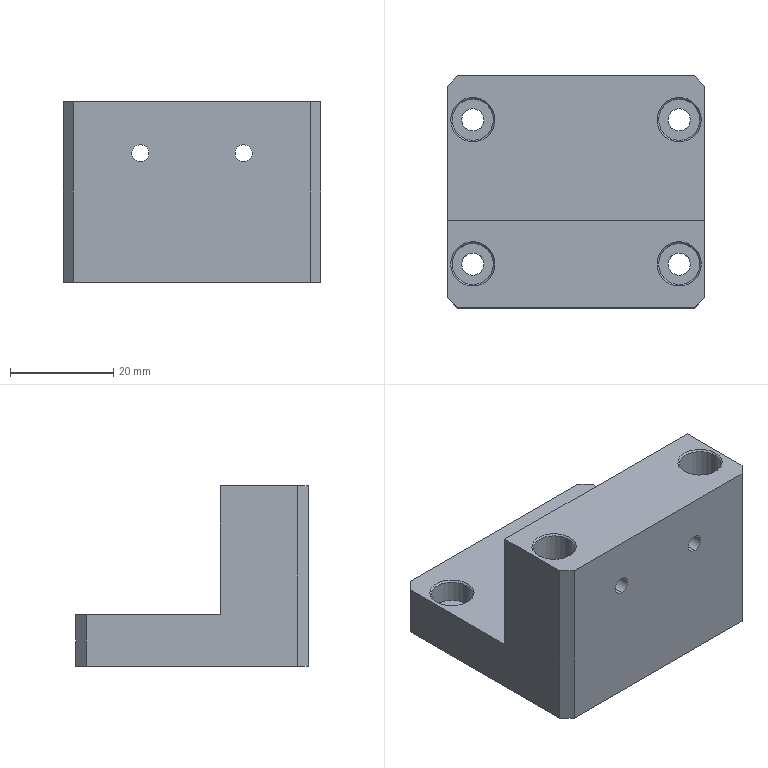Part | SolidWorks | features HoleWzd 3, Chamfer 1, Extrusion 1, ICE 1 | 1 solid | 48 faces | box 50 x 45 x 35 mm | volume 39850 mm3 | cylinder 20 | plane 16 | cone 12 | commonest cylinder face diameters 4.3 x8 8 x8 3.3 x4
STEP:
#1=CARTESIAN_POINT('',(-35.,16.625,23.35));
#2=VERTEX_POINT('',#1);
#3=CARTESIAN_POINT('',(-35.,16.625,26.65));
#4=VERTEX_POINT('',#3);
#5=CARTESIAN_POINT('',(-35.,16.625,25.));
#6=DIRECTION('',(0.,1.,0.));
#7=DIRECTION('',(0.,0.,1.));
#8=AXIS2_PLACEMENT_3D('',#5,#6,#7);
#9=CIRCLE('',#8,1.65);
#10=EDGE_CURVE('',#2,#4,#9,.T.);
#11=ORIENTED_EDGE('',*,*,#10,.F.);
#12=CARTESIAN_POINT('',(-35.,17.,22.975));
#13=VERTEX_POINT('',#12);
#14=CARTESIAN_POINT('',(-35.,17.,22.975));
#15=DIRECTION('',(0.,0.7071,-0.7071));
#16=VECTOR('',#15,1000.);
#17=LINE('',#14,#16);
#18=EDGE_CURVE('',#2,#13,#17,.T.);
#19=ORIENTED_EDGE('',*,*,#18,.T.);
#20=CARTESIAN_POINT('',(-35.,17.,27.025));
#21=VERTEX_POINT('',#20);
#22=CARTESIAN_POINT('',(-35.,17.,25.));
#23=DIRECTION('',(0.,1.,0.));
#24=DIRECTION('',(0.,0.,1.));
#25=AXIS2_PLACEMENT_3D('',#22,#23,#24);
#26=CIRCLE('',#25,2.025);
#27=EDGE_CURVE('',#13,#21,#26,.T.);
#28=ORIENTED_EDGE('',*,*,#27,.T.);
#29=CARTESIAN_POINT('',(-35.,17.,27.025));
#30=DIRECTION('',(0.,0.7071,0.7071));
#31=VECTOR('',#30,1000.);
#32=LINE('',#29,#31);
#33=EDGE_CURVE('',#4,#21,#32,.T.);
#34=ORIENTED_EDGE('',*,*,#33,.F.);
#35=EDGE_LOOP('',(#11,#19,#28,#34));
#36=FACE_OUTER_BOUND('',#35,.T.);
#37=CARTESIAN_POINT('',(-35.,17.,25.));
#38=DIRECTION('',(0.,1.,0.));
#39=DIRECTION('',(0.,0.,1.));
#40=AXIS2_PLACEMENT_3D('',#37,#38,#39);
#41=CONICAL_SURFACE('',#40,2.025,0.7854);
#42=ADVANCED_FACE('',(#36),#41,.F.);
#43=CARTESIAN_POINT('',(-35.,0.,23.35));
#44=VERTEX_POINT('',#43);
#45=CARTESIAN_POINT('',(-35.,0.,26.65));
#46=VERTEX_POINT('',#45);
#47=CARTESIAN_POINT('',(-35.,0.,25.));
#48=DIRECTION('',(0.,1.,0.));
#49=DIRECTION('',(0.,0.,1.));
#50=AXIS2_PLACEMENT_3D('',#47,#48,#49);
#51=CIRCLE('',#50,1.65);
#52=EDGE_CURVE('',#44,#46,#51,.T.);
#53=ORIENTED_EDGE('',*,*,#52,.F.);
#54=CARTESIAN_POINT('',(-35.,17.,23.35));
#55=DIRECTION('',(0.,1.,0.));
#56=VECTOR('',#55,1000.);
#57=LINE('',#54,#56);
#58=EDGE_CURVE('',#44,#2,#57,.T.);
#59=ORIENTED_EDGE('',*,*,#58,.T.);
#60=ORIENTED_EDGE('',*,*,#10,.T.);
#61=CARTESIAN_POINT('',(-35.,17.,26.65));
#62=DIRECTION('',(0.,1.,0.));
#63=VECTOR('',#62,1000.);
#64=LINE('',#61,#63);
#65=EDGE_CURVE('',#46,#4,#64,.T.);
#66=ORIENTED_EDGE('',*,*,#65,.F.);
#67=EDGE_LOOP('',(#53,#59,#60,#66));
#68=FACE_OUTER_BOUND('',#67,.T.);
#69=CARTESIAN_POINT('',(-35.,17.,25.));
#70=DIRECTION('',(0.,1.,0.));
#71=DIRECTION('',(0.,0.,1.));
#72=AXIS2_PLACEMENT_3D('',#69,#70,#71);
#73=CYLINDRICAL_SURFACE('',#72,1.65);
#74=ADVANCED_FACE('',(#68),#73,.F.);
#75=CARTESIAN_POINT('',(-15.,16.625,23.35));
#76=VERTEX_POINT('',#75);
#77=CARTESIAN_POINT('',(-15.,16.625,26.65));
#78=VERTEX_POINT('',#77);
#79=CARTESIAN_POINT('',(-15.,16.625,25.));
#80=DIRECTION('',(0.,1.,0.));
#81=DIRECTION('',(0.,0.,1.));
#82=AXIS2_PLACEMENT_3D('',#79,#80,#81);
#83=CIRCLE('',#82,1.65);
#84=EDGE_CURVE('',#76,#78,#83,.T.);
#85=ORIENTED_EDGE('',*,*,#84,.F.);
#86=CARTESIAN_POINT('',(-15.,17.,22.975));
#87=VERTEX_POINT('',#86);
#88=CARTESIAN_POINT('',(-15.,17.,22.975));
#89=DIRECTION('',(0.,0.7071,-0.7071));
#90=VECTOR('',#89,1000.);
#91=LINE('',#88,#90);
#92=EDGE_CURVE('',#76,#87,#91,.T.);
#93=ORIENTED_EDGE('',*,*,#92,.T.);
#94=CARTESIAN_POINT('',(-15.,17.,27.025));
#95=VERTEX_POINT('',#94);
#96=CARTESIAN_POINT('',(-15.,17.,25.));
#97=DIRECTION('',(0.,1.,0.));
#98=DIRECTION('',(0.,0.,1.));
#99=AXIS2_PLACEMENT_3D('',#96,#97,#98);
#100=CIRCLE('',#99,2.025);
#101=EDGE_CURVE('',#87,#95,#100,.T.);
#102=ORIENTED_EDGE('',*,*,#101,.T.);
#103=CARTESIAN_POINT('',(-15.,17.,27.025));
#104=DIRECTION('',(0.,0.7071,0.7071));
#105=VECTOR('',#104,1000.);
#106=LINE('',#103,#105);
#107=EDGE_CURVE('',#78,#95,#106,.T.);
#108=ORIENTED_EDGE('',*,*,#107,.F.);
#109=EDGE_LOOP('',(#85,#93,#102,#108));
#110=FACE_OUTER_BOUND('',#109,.T.);
#111=CARTESIAN_POINT('',(-15.,17.,25.));
#112=DIRECTION('',(0.,1.,0.));
#113=DIRECTION('',(0.,0.,1.));
#114=AXIS2_PLACEMENT_3D('',#111,#112,#113);
#115=CONICAL_SURFACE('',#114,2.025,0.7854);
#116=ADVANCED_FACE('',(#110),#115,.F.);
#117=CARTESIAN_POINT('',(-15.,0.,23.35));
#118=VERTEX_POINT('',#117);
#119=CARTESIAN_POINT('',(-15.,0.,26.65));
#120=VERTEX_POINT('',#119);
#121=CARTESIAN_POINT('',(-15.,0.,25.));
#122=DIRECTION('',(0.,1.,0.));
#123=DIRECTION('',(0.,0.,1.));
#124=AXIS2_PLACEMENT_3D('',#121,#122,#123);
#125=CIRCLE('',#124,1.65);
#126=EDGE_CURVE('',#118,#120,#125,.T.);
#127=ORIENTED_EDGE('',*,*,#126,.F.);
#128=CARTESIAN_POINT('',(-15.,17.,23.35));
#129=DIRECTION('',(0.,1.,0.));
#130=VECTOR('',#129,1000.);
#131=LINE('',#128,#130);
#132=EDGE_CURVE('',#118,#76,#131,.T.);
#133=ORIENTED_EDGE('',*,*,#132,.T.);
#134=ORIENTED_EDGE('',*,*,#84,.T.);
#135=CARTESIAN_POINT('',(-15.,17.,26.65));
#136=DIRECTION('',(0.,1.,0.));
#137=VECTOR('',#136,1000.);
#138=LINE('',#135,#137);
#139=EDGE_CURVE('',#120,#78,#138,.T.);
#140=ORIENTED_EDGE('',*,*,#139,.F.);
#141=EDGE_LOOP('',(#127,#133,#134,#140));
#142=FACE_OUTER_BOUND('',#141,.T.);
#143=CARTESIAN_POINT('',(-15.,17.,25.));
#144=DIRECTION('',(0.,1.,0.));
#145=DIRECTION('',(0.,0.,1.));
#146=AXIS2_PLACEMENT_3D('',#143,#144,#145);
#147=CYLINDRICAL_SURFACE('',#146,1.65);
#148=ADVANCED_FACE('',(#142),#147,.F.);
#149=CARTESIAN_POINT('',(-49.,8.5,34.7));
#150=VERTEX_POINT('',#149);
#151=CARTESIAN_POINT('',(-41.,8.5,34.7));
#152=VERTEX_POINT('',#151);
#153=CARTESIAN_POINT('',(-45.,8.5,34.7));
#154=DIRECTION('',(0.,0.,1.));
#155=DIRECTION('',(1.,0.,0.));
#156=AXIS2_PLACEMENT_3D('',#153,#154,#155);
#157=CIRCLE('',#156,4.);
#158=EDGE_CURVE('',#150,#152,#157,.T.);
#159=ORIENTED_EDGE('',*,*,#158,.F.);
#160=CARTESIAN_POINT('',(-49.3,8.5,35.));
#161=VERTEX_POINT('',#160);
#162=CARTESIAN_POINT('',(-49.3,8.5,35.));
#163=DIRECTION('',(-0.7071,0.,0.7071));
#164=VECTOR('',#163,1000.);
#165=LINE('',#162,#164);
#166=EDGE_CURVE('',#150,#161,#165,.T.);
#167=ORIENTED_EDGE('',*,*,#166,.T.);
#168=CARTESIAN_POINT('',(-40.7,8.5,35.));
#169=VERTEX_POINT('',#168);
#170=CARTESIAN_POINT('',(-45.,8.5,35.));
#171=DIRECTION('',(0.,0.,1.));
#172=DIRECTION('',(1.,0.,0.));
#173=AXIS2_PLACEMENT_3D('',#170,#171,#172);
#174=CIRCLE('',#173,4.3);
#175=EDGE_CURVE('',#161,#169,#174,.T.);
#176=ORIENTED_EDGE('',*,*,#175,.T.);
#177=CARTESIAN_POINT('',(-40.7,8.5,35.));
#178=DIRECTION('',(0.7071,0.,0.7071));
#179=VECTOR('',#178,1000.);
#180=LINE('',#177,#179);
#181=EDGE_CURVE('',#152,#169,#180,.T.);
#182=ORIENTED_EDGE('',*,*,#181,.F.);
#183=EDGE_LOOP('',(#159,#167,#176,#182));
#184=FACE_OUTER_BOUND('',#183,.T.);
#185=CARTESIAN_POINT('',(-45.,8.5,35.));
#186=DIRECTION('',(0.,0.,1.));
#187=DIRECTION('',(1.,0.,0.));
#188=AXIS2_PLACEMENT_3D('',#185,#186,#187);
#189=CONICAL_SURFACE('',#188,4.3,0.7854);
#190=ADVANCED_FACE('',(#184),#189,.F.);
#191=CARTESIAN_POINT('',(-49.,8.5,10.));
#192=VERTEX_POINT('',#191);
#193=CARTESIAN_POINT('',(-41.,8.5,10.));
#194=VERTEX_POINT('',#193);
#195=CARTESIAN_POINT('',(-45.,8.5,10.));
#196=DIRECTION('',(0.,0.,1.));
#197=DIRECTION('',(1.,0.,0.));
#198=AXIS2_PLACEMENT_3D('',#195,#196,#197);
#199=CIRCLE('',#198,4.);
#200=EDGE_CURVE('',#192,#194,#199,.T.);
#201=ORIENTED_EDGE('',*,*,#200,.F.);
#202=CARTESIAN_POINT('',(-49.,8.5,35.));
#203=DIRECTION('',(0.,0.,1.));
#204=VECTOR('',#203,1000.);
#205=LINE('',#202,#204);
#206=EDGE_CURVE('',#192,#150,#205,.T.);
#207=ORIENTED_EDGE('',*,*,#206,.T.);
#208=ORIENTED_EDGE('',*,*,#158,.T.);
#209=CARTESIAN_POINT('',(-41.,8.5,35.));
#210=DIRECTION('',(0.,0.,1.));
#211=VECTOR('',#210,1000.);
#212=LINE('',#209,#211);
#213=EDGE_CURVE('',#194,#152,#212,.T.);
#214=ORIENTED_EDGE('',*,*,#213,.F.);
#215=EDGE_LOOP('',(#201,#207,#208,#214));
#216=FACE_OUTER_BOUND('',#215,.T.);
#217=CARTESIAN_POINT('',(-45.,8.5,35.));
#218=DIRECTION('',(0.,0.,1.));
#219=DIRECTION('',(1.,0.,0.));
#220=AXIS2_PLACEMENT_3D('',#217,#218,#219);
#221=CYLINDRICAL_SURFACE('',#220,4.);
#222=ADVANCED_FACE('',(#216),#221,.F.);
#223=CARTESIAN_POINT('',(-47.15,8.5,0.));
#224=VERTEX_POINT('',#223);
#225=CARTESIAN_POINT('',(-42.85,8.5,0.));
#226=VERTEX_POINT('',#225);
#227=CARTESIAN_POINT('',(-45.,8.5,0.));
#228=DIRECTION('',(0.,0.,1.));
#229=DIRECTION('',(1.,0.,0.));
#230=AXIS2_PLACEMENT_3D('',#227,#228,#229);
#231=CIRCLE('',#230,2.15);
#232=EDGE_CURVE('',#224,#226,#231,.T.);
#233=ORIENTED_EDGE('',*,*,#232,.F.);
#234=CARTESIAN_POINT('',(-47.15,8.5,10.));
#235=VERTEX_POINT('',#234);
#236=CARTESIAN_POINT('',(-47.15,8.5,35.));
#237=DIRECTION('',(0.,0.,1.));
#238=VECTOR('',#237,1000.);
#239=LINE('',#236,#238);
#240=EDGE_CURVE('',#224,#235,#239,.T.);
#241=ORIENTED_EDGE('',*,*,#240,.T.);
#242=CARTESIAN_POINT('',(-42.85,8.5,10.));
#243=VERTEX_POINT('',#242);
#244=CARTESIAN_POINT('',(-45.,8.5,10.));
#245=DIRECTION('',(0.,0.,1.));
#246=DIRECTION('',(1.,0.,0.));
#247=AXIS2_PLACEMENT_3D('',#244,#245,#246);
#248=CIRCLE('',#247,2.15);
#249=EDGE_CURVE('',#235,#243,#248,.T.);
#250=ORIENTED_EDGE('',*,*,#249,.T.);
#251=CARTESIAN_POINT('',(-42.85,8.5,35.));
#252=DIRECTION('',(0.,0.,1.));
#253=VECTOR('',#252,1000.);
#254=LINE('',#251,#253);
#255=EDGE_CURVE('',#226,#243,#254,.T.);
#256=ORIENTED_EDGE('',*,*,#255,.F.);
#257=EDGE_LOOP('',(#233,#241,#250,#256));
#258=FACE_OUTER_BOUND('',#257,.T.);
#259=CARTESIAN_POINT('',(-45.,8.5,35.));
#260=DIRECTION('',(0.,0.,1.));
#261=DIRECTION('',(1.,0.,0.));
#262=AXIS2_PLACEMENT_3D('',#259,#260,#261);
#263=CYLINDRICAL_SURFACE('',#262,2.15);
#264=ADVANCED_FACE('',(#258),#263,.F.);
#265=CARTESIAN_POINT('',(-9.,8.5,34.7));
#266=VERTEX_POINT('',#265);
#267=CARTESIAN_POINT('',(-1.,8.5,34.7));
#268=VERTEX_POINT('',#267);
#269=CARTESIAN_POINT('',(-5.,8.5,34.7));
#270=DIRECTION('',(0.,0.,1.));
#271=DIRECTION('',(1.,0.,0.));
#272=AXIS2_PLACEMENT_3D('',#269,#270,#271);
#273=CIRCLE('',#272,4.);
#274=EDGE_CURVE('',#266,#268,#273,.T.);
#275=ORIENTED_EDGE('',*,*,#274,.F.);
#276=CARTESIAN_POINT('',(-9.3,8.5,35.));
#277=VERTEX_POINT('',#276);
#278=CARTESIAN_POINT('',(-9.3,8.5,35.));
#279=DIRECTION('',(-0.7071,0.,0.7071));
#280=VECTOR('',#279,1000.);
#281=LINE('',#278,#280);
#282=EDGE_CURVE('',#266,#277,#281,.T.);
#283=ORIENTED_EDGE('',*,*,#282,.T.);
#284=CARTESIAN_POINT('',(-0.7,8.5,35.));
#285=VERTEX_POINT('',#284);
#286=CARTESIAN_POINT('',(-5.,8.5,35.));
#287=DIRECTION('',(0.,0.,1.));
#288=DIRECTION('',(1.,0.,0.));
#289=AXIS2_PLACEMENT_3D('',#286,#287,#288);
#290=CIRCLE('',#289,4.3);
#291=EDGE_CURVE('',#277,#285,#290,.T.);
#292=ORIENTED_EDGE('',*,*,#291,.T.);
#293=CARTESIAN_POINT('',(-0.7,8.5,35.));
#294=DIRECTION('',(0.7071,0.,0.7071));
#295=VECTOR('',#294,1000.);
#296=LINE('',#293,#295);
#297=EDGE_CURVE('',#268,#285,#296,.T.);
#298=ORIENTED_EDGE('',*,*,#297,.F.);
#299=EDGE_LOOP('',(#275,#283,#292,#298));
#300=FACE_OUTER_BOUND('',#299,.T.);
#301=CARTESIAN_POINT('',(-5.,8.5,35.));
#302=DIRECTION('',(0.,0.,1.));
#303=DIRECTION('',(1.,0.,0.));
#304=AXIS2_PLACEMENT_3D('',#301,#302,#303);
#305=CONICAL_SURFACE('',#304,4.3,0.7854);
#306=ADVANCED_FACE('',(#300),#305,.F.);
#307=CARTESIAN_POINT('',(-9.,8.5,10.));
#308=VERTEX_POINT('',#307);
#309=CARTESIAN_POINT('',(-1.,8.5,10.));
#310=VERTEX_POINT('',#309);
#311=CARTESIAN_POINT('',(-5.,8.5,10.));
#312=DIRECTION('',(0.,0.,1.));
#313=DIRECTION('',(1.,0.,0.));
#314=AXIS2_PLACEMENT_3D('',#311,#312,#313);
#315=CIRCLE('',#314,4.);
#316=EDGE_CURVE('',#308,#310,#315,.T.);
#317=ORIENTED_EDGE('',*,*,#316,.F.);
#318=CARTESIAN_POINT('',(-9.,8.5,35.));
#319=DIRECTION('',(0.,0.,1.));
#320=VECTOR('',#319,1000.);
#321=LINE('',#318,#320);
#322=EDGE_CURVE('',#308,#266,#321,.T.);
#323=ORIENTED_EDGE('',*,*,#322,.T.);
#324=ORIENTED_EDGE('',*,*,#274,.T.);
#325=CARTESIAN_POINT('',(-1.,8.5,35.));
#326=DIRECTION('',(0.,0.,1.));
#327=VECTOR('',#326,1000.);
#328=LINE('',#325,#327);
#329=EDGE_CURVE('',#310,#268,#328,.T.);
#330=ORIENTED_EDGE('',*,*,#329,.F.);
#331=EDGE_LOOP('',(#317,#323,#324,#330));
#332=FACE_OUTER_BOUND('',#331,.T.);
#333=CARTESIAN_POINT('',(-5.,8.5,35.));
#334=DIRECTION('',(0.,0.,1.));
#335=DIRECTION('',(1.,0.,0.));
#336=AXIS2_PLACEMENT_3D('',#333,#334,#335);
#337=CYLINDRICAL_SURFACE('',#336,4.);
#338=ADVANCED_FACE('',(#332),#337,.F.);
#339=CARTESIAN_POINT('',(-7.15,8.5,0.));
#340=VERTEX_POINT('',#339);
#341=CARTESIAN_POINT('',(-2.85,8.5,0.));
#342=VERTEX_POINT('',#341);
#343=CARTESIAN_POINT('',(-5.,8.5,0.));
#344=DIRECTION('',(0.,0.,1.));
#345=DIRECTION('',(1.,0.,0.));
#346=AXIS2_PLACEMENT_3D('',#343,#344,#345);
#347=CIRCLE('',#346,2.15);
#348=EDGE_CURVE('',#340,#342,#347,.T.);
#349=ORIENTED_EDGE('',*,*,#348,.F.);
#350=CARTESIAN_POINT('',(-7.15,8.5,10.));
#351=VERTEX_POINT('',#350);
#352=CARTESIAN_POINT('',(-7.15,8.5,35.));
#353=DIRECTION('',(0.,0.,1.));
#354=VECTOR('',#353,1000.);
#355=LINE('',#352,#354);
#356=EDGE_CURVE('',#340,#351,#355,.T.);
#357=ORIENTED_EDGE('',*,*,#356,.T.);
#358=CARTESIAN_POINT('',(-2.85,8.5,10.));
#359=VERTEX_POINT('',#358);
#360=CARTESIAN_POINT('',(-5.,8.5,10.));
#361=DIRECTION('',(0.,0.,1.));
#362=DIRECTION('',(1.,0.,0.));
#363=AXIS2_PLACEMENT_3D('',#360,#361,#362);
#364=CIRCLE('',#363,2.15);
#365=EDGE_CURVE('',#351,#359,#364,.T.);
#366=ORIENTED_EDGE('',*,*,#365,.T.);
#367=CARTESIAN_POINT('',(-2.85,8.5,35.));
#368=DIRECTION('',(0.,0.,1.));
#369=VECTOR('',#368,1000.);
#370=LINE('',#367,#369);
#371=EDGE_CURVE('',#342,#359,#370,.T.);
#372=ORIENTED_EDGE('',*,*,#371,.F.);
#373=EDGE_LOOP('',(#349,#357,#366,#372));
#374=FACE_OUTER_BOUND('',#373,.T.);
#375=CARTESIAN_POINT('',(-5.,8.5,35.));
#376=DIRECTION('',(0.,0.,1.));
#377=DIRECTION('',(1.,0.,0.));
#378=AXIS2_PLACEMENT_3D('',#375,#376,#377);
#379=CYLINDRICAL_SURFACE('',#378,2.15);
#380=ADVANCED_FACE('',(#374),#379,.F.);
#381=CARTESIAN_POINT('',(-49.,36.5,9.7));
#382=VERTEX_POINT('',#381);
#383=CARTESIAN_POINT('',(-41.,36.5,9.7));
#384=VERTEX_POINT('',#383);
#385=CARTESIAN_POINT('',(-45.,36.5,9.7));
#386=DIRECTION('',(0.,0.,1.));
#387=DIRECTION('',(1.,0.,0.));
#388=AXIS2_PLACEMENT_3D('',#385,#386,#387);
#389=CIRCLE('',#388,4.);
#390=EDGE_CURVE('',#382,#384,#389,.T.);
#391=ORIENTED_EDGE('',*,*,#390,.F.);
#392=CARTESIAN_POINT('',(-49.3,36.5,10.));
#393=VERTEX_POINT('',#392);
#394=CARTESIAN_POINT('',(-49.3,36.5,10.));
#395=DIRECTION('',(-0.7071,0.,0.7071));
#396=VECTOR('',#395,1000.);
#397=LINE('',#394,#396);
#398=EDGE_CURVE('',#382,#393,#397,.T.);
#399=ORIENTED_EDGE('',*,*,#398,.T.);
#400=CARTESIAN_POINT('',(-40.7,36.5,10.));
#401=VERTEX_POINT('',#400);
#402=CARTESIAN_POINT('',(-45.,36.5,10.));
#403=DIRECTION('',(0.,0.,1.));
#404=DIRECTION('',(1.,0.,0.));
#405=AXIS2_PLACEMENT_3D('',#402,#403,#404);
#406=CIRCLE('',#405,4.3);
#407=EDGE_CURVE('',#393,#401,#406,.T.);
#408=ORIENTED_EDGE('',*,*,#407,.T.);
#409=CARTESIAN_POINT('',(-40.7,36.5,10.));
#410=DIRECTION('',(0.7071,0.,0.7071));
#411=VECTOR('',#410,1000.);
#412=LINE('',#409,#411);
#413=EDGE_CURVE('',#384,#401,#412,.T.);
#414=ORIENTED_EDGE('',*,*,#413,.F.);
#415=EDGE_LOOP('',(#391,#399,#408,#414));
#416=FACE_OUTER_BOUND('',#415,.T.);
#417=CARTESIAN_POINT('',(-45.,36.5,10.));
#418=DIRECTION('',(0.,0.,1.));
#419=DIRECTION('',(1.,0.,0.));
#420=AXIS2_PLACEMENT_3D('',#417,#418,#419);
#421=CONICAL_SURFACE('',#420,4.3,0.7854);
#422=ADVANCED_FACE('',(#416),#421,.F.);
#423=CARTESIAN_POINT('',(-49.,36.5,5.4));
#424=VERTEX_POINT('',#423);
#425=CARTESIAN_POINT('',(-41.,36.5,5.4));
#426=VERTEX_POINT('',#425);
#427=CARTESIAN_POINT('',(-45.,36.5,5.4));
#428=DIRECTION('',(0.,0.,1.));
#429=DIRECTION('',(1.,0.,0.));
#430=AXIS2_PLACEMENT_3D('',#427,#428,#429);
#431=CIRCLE('',#430,4.);
#432=EDGE_CURVE('',#424,#426,#431,.T.);
#433=ORIENTED_EDGE('',*,*,#432,.F.);
#434=CARTESIAN_POINT('',(-49.,36.5,10.));
#435=DIRECTION('',(0.,0.,1.));
#436=VECTOR('',#435,1000.);
#437=LINE('',#434,#436);
#438=EDGE_CURVE('',#424,#382,#437,.T.);
#439=ORIENTED_EDGE('',*,*,#438,.T.);
#440=ORIENTED_EDGE('',*,*,#390,.T.);
#441=CARTESIAN_POINT('',(-41.,36.5,10.));
#442=DIRECTION('',(0.,0.,1.));
#443=VECTOR('',#442,1000.);
#444=LINE('',#441,#443);
#445=EDGE_CURVE('',#426,#384,#444,.T.);
#446=ORIENTED_EDGE('',*,*,#445,.F.);
#447=EDGE_LOOP('',(#433,#439,#440,#446));
#448=FACE_OUTER_BOUND('',#447,.T.);
#449=CARTESIAN_POINT('',(-45.,36.5,10.));
#450=DIRECTION('',(0.,0.,1.));
#451=DIRECTION('',(1.,0.,0.));
#452=AXIS2_PLACEMENT_3D('',#449,#450,#451);
#453=CYLINDRICAL_SURFACE('',#452,4.);
#454=ADVANCED_FACE('',(#448),#453,.F.);
#455=CARTESIAN_POINT('',(-47.15,36.5,0.));
#456=VERTEX_POINT('',#455);
#457=CARTESIAN_POINT('',(-42.85,36.5,0.));
#458=VERTEX_POINT('',#457);
#459=CARTESIAN_POINT('',(-45.,36.5,0.));
#460=DIRECTION('',(0.,0.,1.));
#461=DIRECTION('',(1.,0.,0.));
#462=AXIS2_PLACEMENT_3D('',#459,#460,#461);
#463=CIRCLE('',#462,2.15);
#464=EDGE_CURVE('',#456,#458,#463,.T.);
#465=ORIENTED_EDGE('',*,*,#464,.F.);
#466=CARTESIAN_POINT('',(-47.15,36.5,5.4));
#467=VERTEX_POINT('',#466);
#468=CARTESIAN_POINT('',(-47.15,36.5,10.));
#469=DIRECTION('',(0.,0.,1.));
#470=VECTOR('',#469,1000.);
#471=LINE('',#468,#470);
#472=EDGE_CURVE('',#456,#467,#471,.T.);
#473=ORIENTED_EDGE('',*,*,#472,.T.);
#474=CARTESIAN_POINT('',(-42.85,36.5,5.4));
#475=VERTEX_POINT('',#474);
#476=CARTESIAN_POINT('',(-45.,36.5,5.4));
#477=DIRECTION('',(0.,0.,1.));
#478=DIRECTION('',(1.,0.,0.));
#479=AXIS2_PLACEMENT_3D('',#476,#477,#478);
#480=CIRCLE('',#479,2.15);
#481=EDGE_CURVE('',#467,#475,#480,.T.);
#482=ORIENTED_EDGE('',*,*,#481,.T.);
#483=CARTESIAN_POINT('',(-42.85,36.5,10.));
#484=DIRECTION('',(0.,0.,1.));
#485=VECTOR('',#484,1000.);
#486=LINE('',#483,#485);
#487=EDGE_CURVE('',#458,#475,#486,.T.);
#488=ORIENTED_EDGE('',*,*,#487,.F.);
#489=EDGE_LOOP('',(#465,#473,#482,#488));
#490=FACE_OUTER_BOUND('',#489,.T.);
#491=CARTESIAN_POINT('',(-45.,36.5,10.));
#492=DIRECTION('',(0.,0.,1.));
#493=DIRECTION('',(1.,0.,0.));
#494=AXIS2_PLACEMENT_3D('',#491,#492,#493);
#495=CYLINDRICAL_SURFACE('',#494,2.15);
#496=ADVANCED_FACE('',(#490),#495,.F.);
#497=CARTESIAN_POINT('',(-9.,36.5,9.7));
#498=VERTEX_POINT('',#497);
#499=CARTESIAN_POINT('',(-1.,36.5,9.7));
#500=VERTEX_POINT('',#499);
#501=CARTESIAN_POINT('',(-5.,36.5,9.7));
#502=DIRECTION('',(0.,0.,1.));
#503=DIRECTION('',(1.,0.,0.));
#504=AXIS2_PLACEMENT_3D('',#501,#502,#503);
#505=CIRCLE('',#504,4.);
#506=EDGE_CURVE('',#498,#500,#505,.T.);
#507=ORIENTED_EDGE('',*,*,#506,.F.);
#508=CARTESIAN_POINT('',(-9.3,36.5,10.));
#509=VERTEX_POINT('',#508);
#510=CARTESIAN_POINT('',(-9.3,36.5,10.));
#511=DIRECTION('',(-0.7071,0.,0.7071));
#512=VECTOR('',#511,1000.);
#513=LINE('',#510,#512);
#514=EDGE_CURVE('',#498,#509,#513,.T.);
#515=ORIENTED_EDGE('',*,*,#514,.T.);
#516=CARTESIAN_POINT('',(-0.7,36.5,10.));
#517=VERTEX_POINT('',#516);
#518=CARTESIAN_POINT('',(-5.,36.5,10.));
#519=DIRECTION('',(0.,0.,1.));
#520=DIRECTION('',(1.,0.,0.));
#521=AXIS2_PLACEMENT_3D('',#518,#519,#520);
#522=CIRCLE('',#521,4.3);
#523=EDGE_CURVE('',#509,#517,#522,.T.);
#524=ORIENTED_EDGE('',*,*,#523,.T.);
#525=CARTESIAN_POINT('',(-0.7,36.5,10.));
#526=DIRECTION('',(0.7071,0.,0.7071));
#527=VECTOR('',#526,1000.);
#528=LINE('',#525,#527);
#529=EDGE_CURVE('',#500,#517,#528,.T.);
#530=ORIENTED_EDGE('',*,*,#529,.F.);
#531=EDGE_LOOP('',(#507,#515,#524,#530));
#532=FACE_OUTER_BOUND('',#531,.T.);
#533=CARTESIAN_POINT('',(-5.,36.5,10.));
#534=DIRECTION('',(0.,0.,1.));
#535=DIRECTION('',(1.,0.,0.));
#536=AXIS2_PLACEMENT_3D('',#533,#534,#535);
#537=CONICAL_SURFACE('',#536,4.3,0.7854);
#538=ADVANCED_FACE('',(#532),#537,.F.);
#539=CARTESIAN_POINT('',(-9.,36.5,5.4));
#540=VERTEX_POINT('',#539);
#541=CARTESIAN_POINT('',(-1.,36.5,5.4));
#542=VERTEX_POINT('',#541);
#543=CARTESIAN_POINT('',(-5.,36.5,5.4));
#544=DIRECTION('',(0.,0.,1.));
#545=DIRECTION('',(1.,0.,0.));
#546=AXIS2_PLACEMENT_3D('',#543,#544,#545);
#547=CIRCLE('',#546,4.);
#548=EDGE_CURVE('',#540,#542,#547,.T.);
#549=ORIENTED_EDGE('',*,*,#548,.F.);
#550=CARTESIAN_POINT('',(-9.,36.5,10.));
#551=DIRECTION('',(0.,0.,1.));
#552=VECTOR('',#551,1000.);
#553=LINE('',#550,#552);
#554=EDGE_CURVE('',#540,#498,#553,.T.);
#555=ORIENTED_EDGE('',*,*,#554,.T.);
#556=ORIENTED_EDGE('',*,*,#506,.T.);
#557=CARTESIAN_POINT('',(-1.,36.5,10.));
#558=DIRECTION('',(0.,0.,1.));
#559=VECTOR('',#558,1000.);
#560=LINE('',#557,#559);
#561=EDGE_CURVE('',#542,#500,#560,.T.);
#562=ORIENTED_EDGE('',*,*,#561,.F.);
#563=EDGE_LOOP('',(#549,#555,#556,#562));
#564=FACE_OUTER_BOUND('',#563,.T.);
#565=CARTESIAN_POINT('',(-5.,36.5,10.));
#566=DIRECTION('',(0.,0.,1.));
#567=DIRECTION('',(1.,0.,0.));
#568=AXIS2_PLACEMENT_3D('',#565,#566,#567);
#569=CYLINDRICAL_SURFACE('',#568,4.);
#570=ADVANCED_FACE('',(#564),#569,.F.);
#571=CARTESIAN_POINT('',(-7.15,36.5,0.));
#572=VERTEX_POINT('',#571);
#573=CARTESIAN_POINT('',(-2.85,36.5,0.));
#574=VERTEX_POINT('',#573);
#575=CARTESIAN_POINT('',(-5.,36.5,0.));
#576=DIRECTION('',(0.,0.,1.));
#577=DIRECTION('',(1.,0.,0.));
#578=AXIS2_PLACEMENT_3D('',#575,#576,#577);
#579=CIRCLE('',#578,2.15);
#580=EDGE_CURVE('',#572,#574,#579,.T.);
#581=ORIENTED_EDGE('',*,*,#580,.F.);
#582=CARTESIAN_POINT('',(-7.15,36.5,5.4));
#583=VERTEX_POINT('',#582);
#584=CARTESIAN_POINT('',(-7.15,36.5,10.));
#585=DIRECTION('',(0.,0.,1.));
#586=VECTOR('',#585,1000.);
#587=LINE('',#584,#586);
#588=EDGE_CURVE('',#572,#583,#587,.T.);
#589=ORIENTED_EDGE('',*,*,#588,.T.);
#590=CARTESIAN_POINT('',(-2.85,36.5,5.4));
#591=VERTEX_POINT('',#590);
#592=CARTESIAN_POINT('',(-5.,36.5,5.4));
#593=DIRECTION('',(0.,0.,1.));
#594=DIRECTION('',(1.,0.,0.));
#595=AXIS2_PLACEMENT_3D('',#592,#593,#594);
#596=CIRCLE('',#595,2.15);
#597=EDGE_CURVE('',#583,#591,#596,.T.);
#598=ORIENTED_EDGE('',*,*,#597,.T.);
#599=CARTESIAN_POINT('',(-2.85,36.5,10.));
#600=DIRECTION('',(0.,0.,1.));
#601=VECTOR('',#600,1000.);
#602=LINE('',#599,#601);
#603=EDGE_CURVE('',#574,#591,#602,.T.);
#604=ORIENTED_EDGE('',*,*,#603,.F.);
#605=EDGE_LOOP('',(#581,#589,#598,#604));
#606=FACE_OUTER_BOUND('',#605,.T.);
#607=CARTESIAN_POINT('',(-5.,36.5,10.));
#608=DIRECTION('',(0.,0.,1.));
#609=DIRECTION('',(1.,0.,0.));
#610=AXIS2_PLACEMENT_3D('',#607,#608,#609);
#611=CYLINDRICAL_SURFACE('',#610,2.15);
#612=ADVANCED_FACE('',(#606),#611,.F.);
#613=CARTESIAN_POINT('',(0.,2.,35.));
#614=VERTEX_POINT('',#613);
#615=CARTESIAN_POINT('',(0.,17.,35.));
#616=VERTEX_POINT('',#615);
#617=CARTESIAN_POINT('',(0.,17.,35.));
#618=DIRECTION('',(0.,1.,0.));
#619=VECTOR('',#618,1000.);
#620=LINE('',#617,#619);
#621=EDGE_CURVE('',#614,#616,#620,.T.);
#622=ORIENTED_EDGE('',*,*,#621,.F.);
#623=CARTESIAN_POINT('',(0.,2.,0.));
#624=VERTEX_POINT('',#623);
#625=CARTESIAN_POINT('',(0.,2.,10.));
#626=DIRECTION('',(0.,0.,-1.));
#627=VECTOR('',#626,1000.);
#628=LINE('',#625,#627);
#629=EDGE_CURVE('',#614,#624,#628,.T.);
#630=ORIENTED_EDGE('',*,*,#629,.T.);
#631=CARTESIAN_POINT('',(0.,43.,0.));
#632=VERTEX_POINT('',#631);
#633=CARTESIAN_POINT('',(0.,0.,0.));
#634=DIRECTION('',(0.,1.,0.));
#635=VECTOR('',#634,1000.);
#636=LINE('',#633,#635);
#637=EDGE_CURVE('',#624,#632,#636,.T.);
#638=ORIENTED_EDGE('',*,*,#637,.T.);
#639=CARTESIAN_POINT('',(0.,43.,10.));
#640=VERTEX_POINT('',#639);
#641=CARTESIAN_POINT('',(0.,43.,10.));
#642=DIRECTION('',(0.,0.,1.));
#643=VECTOR('',#642,1000.);
#644=LINE('',#641,#643);
#645=EDGE_CURVE('',#632,#640,#644,.T.);
#646=ORIENTED_EDGE('',*,*,#645,.T.);
#647=CARTESIAN_POINT('',(0.,17.,10.));
#648=VERTEX_POINT('',#647);
#649=CARTESIAN_POINT('',(0.,0.,10.));
#650=DIRECTION('',(0.,1.,0.));
#651=VECTOR('',#650,1000.);
#652=LINE('',#649,#651);
#653=EDGE_CURVE('',#648,#640,#652,.T.);
#654=ORIENTED_EDGE('',*,*,#653,.F.);
#655=CARTESIAN_POINT('',(0.,17.,35.));
#656=DIRECTION('',(0.,0.,-1.));
#657=VECTOR('',#656,1000.);
#658=LINE('',#655,#657);
#659=EDGE_CURVE('',#616,#648,#658,.T.);
#660=ORIENTED_EDGE('',*,*,#659,.F.);
#661=EDGE_LOOP('',(#622,#630,#638,#646,#654,#660));
#662=FACE_OUTER_BOUND('',#661,.T.);
#663=CARTESIAN_POINT('',(0.,0.,10.));
#664=DIRECTION('',(-1.,0.,0.));
#665=DIRECTION('',(0.,0.,1.));
#666=AXIS2_PLACEMENT_3D('',#663,#664,#665);
#667=PLANE('',#666);
#668=ADVANCED_FACE('',(#662),#667,.F.);
#669=CARTESIAN_POINT('',(-2.,45.,10.));
#670=VERTEX_POINT('',#669);
#671=CARTESIAN_POINT('',(-48.,45.,10.));
#672=VERTEX_POINT('',#671);
#673=CARTESIAN_POINT('',(0.,45.,10.));
#674=DIRECTION('',(-1.,0.,0.));
#675=VECTOR('',#674,1000.);
#676=LINE('',#673,#675);
#677=EDGE_CURVE('',#670,#672,#676,.T.);
#678=ORIENTED_EDGE('',*,*,#677,.F.);
#679=CARTESIAN_POINT('',(-2.,45.,0.));
#680=VERTEX_POINT('',#679);
#681=CARTESIAN_POINT('',(-2.,45.,10.));
#682=DIRECTION('',(0.,0.,-1.));
#683=VECTOR('',#682,1000.);
#684=LINE('',#681,#683);
#685=EDGE_CURVE('',#670,#680,#684,.T.);
#686=ORIENTED_EDGE('',*,*,#685,.T.);
#687=CARTESIAN_POINT('',(-48.,45.,0.));
#688=VERTEX_POINT('',#687);
#689=CARTESIAN_POINT('',(0.,45.,0.));
#690=DIRECTION('',(-1.,0.,0.));
#691=VECTOR('',#690,1000.);
#692=LINE('',#689,#691);
#693=EDGE_CURVE('',#680,#688,#692,.T.);
#694=ORIENTED_EDGE('',*,*,#693,.T.);
#695=CARTESIAN_POINT('',(-48.,45.,10.));
#696=DIRECTION('',(0.,0.,1.));
#697=VECTOR('',#696,1000.);
#698=LINE('',#695,#697);
#699=EDGE_CURVE('',#688,#672,#698,.T.);
#700=ORIENTED_EDGE('',*,*,#699,.T.);
#701=EDGE_LOOP('',(#678,#686,#694,#700));
#702=FACE_OUTER_BOUND('',#701,.T.);
#703=CARTESIAN_POINT('',(0.,45.,10.));
#704=DIRECTION('',(0.,-1.,0.));
#705=DIRECTION('',(1.,0.,0.));
#706=AXIS2_PLACEMENT_3D('',#703,#704,#705);
#707=PLANE('',#706);
#708=ADVANCED_FACE('',(#702),#707,.F.);
#709=CARTESIAN_POINT('',(-50.,43.,0.));
#710=VERTEX_POINT('',#709);
#711=CARTESIAN_POINT('',(-50.,2.,0.));
#712=VERTEX_POINT('',#711);
#713=CARTESIAN_POINT('',(-50.,0.,0.));
#714=DIRECTION('',(0.,-1.,0.));
#715=VECTOR('',#714,1000.);
#716=LINE('',#713,#715);
#717=EDGE_CURVE('',#710,#712,#716,.T.);
#718=ORIENTED_EDGE('',*,*,#717,.T.);
#719=CARTESIAN_POINT('',(-50.,2.,35.));
#720=VERTEX_POINT('',#719);
#721=CARTESIAN_POINT('',(-50.,2.,10.));
#722=DIRECTION('',(0.,0.,1.));
#723=VECTOR('',#722,1000.);
#724=LINE('',#721,#723);
#725=EDGE_CURVE('',#712,#720,#724,.T.);
#726=ORIENTED_EDGE('',*,*,#725,.T.);
#727=CARTESIAN_POINT('',(-50.,17.,35.));
#728=VERTEX_POINT('',#727);
#729=CARTESIAN_POINT('',(-50.,17.,35.));
#730=DIRECTION('',(0.,-1.,0.));
#731=VECTOR('',#730,1000.);
#732=LINE('',#729,#731);
#733=EDGE_CURVE('',#728,#720,#732,.T.);
#734=ORIENTED_EDGE('',*,*,#733,.F.);
#735=CARTESIAN_POINT('',(-50.,17.,10.));
#736=VERTEX_POINT('',#735);
#737=CARTESIAN_POINT('',(-50.,17.,35.));
#738=DIRECTION('',(0.,0.,-1.));
#739=VECTOR('',#738,1000.);
#740=LINE('',#737,#739);
#741=EDGE_CURVE('',#728,#736,#740,.T.);
#742=ORIENTED_EDGE('',*,*,#741,.T.);
#743=CARTESIAN_POINT('',(-50.,43.,10.));
#744=VERTEX_POINT('',#743);
#745=CARTESIAN_POINT('',(-50.,0.,10.));
#746=DIRECTION('',(0.,-1.,0.));
#747=VECTOR('',#746,1000.);
#748=LINE('',#745,#747);
#749=EDGE_CURVE('',#744,#736,#748,.T.);
#750=ORIENTED_EDGE('',*,*,#749,.F.);
#751=CARTESIAN_POINT('',(-50.,43.,10.));
#752=DIRECTION('',(0.,0.,-1.));
#753=VECTOR('',#752,1000.);
#754=LINE('',#751,#753);
#755=EDGE_CURVE('',#744,#710,#754,.T.);
#756=ORIENTED_EDGE('',*,*,#755,.T.);
#757=EDGE_LOOP('',(#718,#726,#734,#742,#750,#756));
#758=FACE_OUTER_BOUND('',#757,.T.);
#759=CARTESIAN_POINT('',(-50.,0.,10.));
#760=DIRECTION('',(1.,0.,0.));
#761=DIRECTION('',(0.,0.,-1.));
#762=AXIS2_PLACEMENT_3D('',#759,#760,#761);
#763=PLANE('',#762);
#764=ADVANCED_FACE('',(#758),#763,.F.);
#765=CARTESIAN_POINT('',(-35.,0.,25.));
#766=DIRECTION('',(0.,1.,0.));
#767=DIRECTION('',(0.,0.,1.));
#768=AXIS2_PLACEMENT_3D('',#765,#766,#767);
#769=CIRCLE('',#768,1.65);
#770=EDGE_CURVE('',#46,#44,#769,.T.);
#771=ORIENTED_EDGE('',*,*,#770,.T.);
#772=ORIENTED_EDGE('',*,*,#52,.T.);
#773=EDGE_LOOP('',(#771,#772));
#774=FACE_BOUND('',#773,.T.);
#775=CARTESIAN_POINT('',(-15.,0.,25.));
#776=DIRECTION('',(0.,1.,0.));
#777=DIRECTION('',(0.,0.,1.));
#778=AXIS2_PLACEMENT_3D('',#775,#776,#777);
#779=CIRCLE('',#778,1.65);
#780=EDGE_CURVE('',#120,#118,#779,.T.);
#781=ORIENTED_EDGE('',*,*,#780,.T.);
#782=ORIENTED_EDGE('',*,*,#126,.T.);
#783=EDGE_LOOP('',(#781,#782));
#784=FACE_BOUND('',#783,.T.);
#785=CARTESIAN_POINT('',(-48.,0.,0.));
#786=VERTEX_POINT('',#785);
#787=CARTESIAN_POINT('',(-2.,0.,0.));
#788=VERTEX_POINT('',#787);
#789=CARTESIAN_POINT('',(0.,0.,0.));
#790=DIRECTION('',(1.,0.,0.));
#791=VECTOR('',#790,1000.);
#792=LINE('',#789,#791);
#793=EDGE_CURVE('',#786,#788,#792,.T.);
#794=ORIENTED_EDGE('',*,*,#793,.T.);
#795=CARTESIAN_POINT('',(-2.,0.,35.));
#796=VERTEX_POINT('',#795);
#797=CARTESIAN_POINT('',(-2.,0.,10.));
#798=DIRECTION('',(0.,0.,1.));
#799=VECTOR('',#798,1000.);
#800=LINE('',#797,#799);
#801=EDGE_CURVE('',#788,#796,#800,.T.);
#802=ORIENTED_EDGE('',*,*,#801,.T.);
#803=CARTESIAN_POINT('',(-48.,0.,35.));
#804=VERTEX_POINT('',#803);
#805=CARTESIAN_POINT('',(-50.,0.,35.));
#806=DIRECTION('',(1.,0.,0.));
#807=VECTOR('',#806,1000.);
#808=LINE('',#805,#807);
#809=EDGE_CURVE('',#804,#796,#808,.T.);
#810=ORIENTED_EDGE('',*,*,#809,.F.);
#811=CARTESIAN_POINT('',(-48.,0.,10.));
#812=DIRECTION('',(0.,0.,-1.));
#813=VECTOR('',#812,1000.);
#814=LINE('',#811,#813);
#815=EDGE_CURVE('',#804,#786,#814,.T.);
#816=ORIENTED_EDGE('',*,*,#815,.T.);
#817=EDGE_LOOP('',(#794,#802,#810,#816));
#818=FACE_OUTER_BOUND('',#817,.T.);
#819=CARTESIAN_POINT('',(0.,0.,10.));
#820=DIRECTION('',(0.,1.,0.));
#821=DIRECTION('',(0.,0.,1.));
#822=AXIS2_PLACEMENT_3D('',#819,#820,#821);
#823=PLANE('',#822);
#824=ADVANCED_FACE('',(#774,#784,#818),#823,.F.);
#825=CARTESIAN_POINT('',(-45.,36.5,10.));
#826=DIRECTION('',(0.,0.,1.));
#827=DIRECTION('',(1.,0.,0.));
#828=AXIS2_PLACEMENT_3D('',#825,#826,#827);
#829=CIRCLE('',#828,4.3);
#830=EDGE_CURVE('',#401,#393,#829,.T.);
#831=ORIENTED_EDGE('',*,*,#830,.F.);
#832=ORIENTED_EDGE('',*,*,#407,.F.);
#833=EDGE_LOOP('',(#831,#832));
#834=FACE_BOUND('',#833,.T.);
#835=CARTESIAN_POINT('',(-5.,36.5,10.));
#836=DIRECTION('',(0.,0.,1.));
#837=DIRECTION('',(1.,0.,0.));
#838=AXIS2_PLACEMENT_3D('',#835,#836,#837);
#839=CIRCLE('',#838,4.3);
#840=EDGE_CURVE('',#517,#509,#839,.T.);
#841=ORIENTED_EDGE('',*,*,#840,.F.);
#842=ORIENTED_EDGE('',*,*,#523,.F.);
#843=EDGE_LOOP('',(#841,#842));
#844=FACE_BOUND('',#843,.T.);
#845=ORIENTED_EDGE('',*,*,#653,.T.);
#846=CARTESIAN_POINT('',(21.5,21.5,10.));
#847=DIRECTION('',(-0.7071,0.7071,0.));
#848=VECTOR('',#847,1000.);
#849=LINE('',#846,#848);
#850=EDGE_CURVE('',#640,#670,#849,.T.);
#851=ORIENTED_EDGE('',*,*,#850,.T.);
#852=ORIENTED_EDGE('',*,*,#677,.T.);
#853=CARTESIAN_POINT('',(-46.5,46.5,10.));
#854=DIRECTION('',(-0.7071,-0.7071,0.));
#855=VECTOR('',#854,1000.);
#856=LINE('',#853,#855);
#857=EDGE_CURVE('',#672,#744,#856,.T.);
#858=ORIENTED_EDGE('',*,*,#857,.T.);
#859=ORIENTED_EDGE('',*,*,#749,.T.);
#860=CARTESIAN_POINT('',(-50.,17.,10.));
#861=DIRECTION('',(-1.,0.,0.));
#862=VECTOR('',#861,1000.);
#863=LINE('',#860,#862);
#864=EDGE_CURVE('',#648,#736,#863,.T.);
#865=ORIENTED_EDGE('',*,*,#864,.F.);
#866=EDGE_LOOP('',(#845,#851,#852,#858,#859,#865));
#867=FACE_OUTER_BOUND('',#866,.T.);
#868=CARTESIAN_POINT('',(0.,0.,10.));
#869=DIRECTION('',(0.,0.,1.));
#870=DIRECTION('',(1.,0.,0.));
#871=AXIS2_PLACEMENT_3D('',#868,#869,#870);
#872=PLANE('',#871);
#873=ADVANCED_FACE('',(#834,#844,#867),#872,.T.);
#874=CARTESIAN_POINT('',(-45.,8.5,0.));
#875=DIRECTION('',(0.,0.,1.));
#876=DIRECTION('',(1.,0.,0.));
#877=AXIS2_PLACEMENT_3D('',#874,#875,#876);
#878=CIRCLE('',#877,2.15);
#879=EDGE_CURVE('',#226,#224,#878,.T.);
#880=ORIENTED_EDGE('',*,*,#879,.T.);
#881=ORIENTED_EDGE('',*,*,#232,.T.);
#882=EDGE_LOOP('',(#880,#881));
#883=FACE_BOUND('',#882,.T.);
#884=CARTESIAN_POINT('',(-5.,8.5,0.));
#885=DIRECTION('',(0.,0.,1.));
#886=DIRECTION('',(1.,0.,0.));
#887=AXIS2_PLACEMENT_3D('',#884,#885,#886);
#888=CIRCLE('',#887,2.15);
#889=EDGE_CURVE('',#342,#340,#888,.T.);
#890=ORIENTED_EDGE('',*,*,#889,.T.);
#891=ORIENTED_EDGE('',*,*,#348,.T.);
#892=EDGE_LOOP('',(#890,#891));
#893=FACE_BOUND('',#892,.T.);
#894=CARTESIAN_POINT('',(-45.,36.5,0.));
#895=DIRECTION('',(0.,0.,1.));
#896=DIRECTION('',(1.,0.,0.));
#897=AXIS2_PLACEMENT_3D('',#894,#895,#896);
#898=CIRCLE('',#897,2.15);
#899=EDGE_CURVE('',#458,#456,#898,.T.);
#900=ORIENTED_EDGE('',*,*,#899,.T.);
#901=ORIENTED_EDGE('',*,*,#464,.T.);
#902=EDGE_LOOP('',(#900,#901));
#903=FACE_BOUND('',#902,.T.);
#904=CARTESIAN_POINT('',(-5.,36.5,0.));
#905=DIRECTION('',(0.,0.,1.));
#906=DIRECTION('',(1.,0.,0.));
#907=AXIS2_PLACEMENT_3D('',#904,#905,#906);
#908=CIRCLE('',#907,2.15);
#909=EDGE_CURVE('',#574,#572,#908,.T.);
#910=ORIENTED_EDGE('',*,*,#909,.T.);
#911=ORIENTED_EDGE('',*,*,#580,.T.);
#912=EDGE_LOOP('',(#910,#911));
#913=FACE_BOUND('',#912,.T.);
#914=ORIENTED_EDGE('',*,*,#637,.F.);
#915=CARTESIAN_POINT('',(0.,2.,0.));
#916=DIRECTION('',(-0.7071,-0.7071,0.));
#917=VECTOR('',#916,1000.);
#918=LINE('',#915,#917);
#919=EDGE_CURVE('',#624,#788,#918,.T.);
#920=ORIENTED_EDGE('',*,*,#919,.T.);
#921=ORIENTED_EDGE('',*,*,#793,.F.);
#922=CARTESIAN_POINT('',(-48.,0.,0.));
#923=DIRECTION('',(-0.7071,0.7071,0.));
#924=VECTOR('',#923,1000.);
#925=LINE('',#922,#924);
#926=EDGE_CURVE('',#786,#712,#925,.T.);
#927=ORIENTED_EDGE('',*,*,#926,.T.);
#928=ORIENTED_EDGE('',*,*,#717,.F.);
#929=CARTESIAN_POINT('',(-50.,43.,0.));
#930=DIRECTION('',(0.7071,0.7071,0.));
#931=VECTOR('',#930,1000.);
#932=LINE('',#929,#931);
#933=EDGE_CURVE('',#710,#688,#932,.T.);
#934=ORIENTED_EDGE('',*,*,#933,.T.);
#935=ORIENTED_EDGE('',*,*,#693,.F.);
#936=CARTESIAN_POINT('',(-2.,45.,0.));
#937=DIRECTION('',(0.7071,-0.7071,0.));
#938=VECTOR('',#937,1000.);
#939=LINE('',#936,#938);
#940=EDGE_CURVE('',#680,#632,#939,.T.);
#941=ORIENTED_EDGE('',*,*,#940,.T.);
#942=EDGE_LOOP('',(#914,#920,#921,#927,#928,#934,#935,#941));
#943=FACE_OUTER_BOUND('',#942,.T.);
#944=CARTESIAN_POINT('',(0.,0.,0.));
#945=DIRECTION('',(0.,0.,1.));
#946=DIRECTION('',(1.,0.,0.));
#947=AXIS2_PLACEMENT_3D('',#944,#945,#946);
#948=PLANE('',#947);
#949=ADVANCED_FACE('',(#883,#893,#903,#913,#943),#948,.F.);
#950=CARTESIAN_POINT('',(-35.,17.,25.));
#951=DIRECTION('',(0.,1.,0.));
#952=DIRECTION('',(0.,0.,1.));
#953=AXIS2_PLACEMENT_3D('',#950,#951,#952);
#954=CIRCLE('',#953,2.025);
#955=EDGE_CURVE('',#21,#13,#954,.T.);
#956=ORIENTED_EDGE('',*,*,#955,.F.);
#957=ORIENTED_EDGE('',*,*,#27,.F.);
#958=EDGE_LOOP('',(#956,#957));
#959=FACE_BOUND('',#958,.T.);
#960=CARTESIAN_POINT('',(-15.,17.,25.));
#961=DIRECTION('',(0.,1.,0.));
#962=DIRECTION('',(0.,0.,1.));
#963=AXIS2_PLACEMENT_3D('',#960,#961,#962);
#964=CIRCLE('',#963,2.025);
#965=EDGE_CURVE('',#95,#87,#964,.T.);
#966=ORIENTED_EDGE('',*,*,#965,.F.);
#967=ORIENTED_EDGE('',*,*,#101,.F.);
#968=EDGE_LOOP('',(#966,#967));
#969=FACE_BOUND('',#968,.T.);
#970=ORIENTED_EDGE('',*,*,#864,.T.);
#971=ORIENTED_EDGE('',*,*,#741,.F.);
#972=CARTESIAN_POINT('',(-50.,17.,35.));
#973=DIRECTION('',(-1.,0.,0.));
#974=VECTOR('',#973,1000.);
#975=LINE('',#972,#974);
#976=EDGE_CURVE('',#616,#728,#975,.T.);
#977=ORIENTED_EDGE('',*,*,#976,.F.);
#978=ORIENTED_EDGE('',*,*,#659,.T.);
#979=EDGE_LOOP('',(#970,#971,#977,#978));
#980=FACE_OUTER_BOUND('',#979,.T.);
#981=CARTESIAN_POINT('',(-50.,17.,35.));
#982=DIRECTION('',(0.,-1.,0.));
#983=DIRECTION('',(0.,0.,-1.));
#984=AXIS2_PLACEMENT_3D('',#981,#982,#983);
#985=PLANE('',#984);
#986=ADVANCED_FACE('',(#959,#969,#980),#985,.F.);
#987=CARTESIAN_POINT('',(-45.,8.5,35.));
#988=DIRECTION('',(0.,0.,1.));
#989=DIRECTION('',(1.,0.,0.));
#990=AXIS2_PLACEMENT_3D('',#987,#988,#989);
#991=CIRCLE('',#990,4.3);
#992=EDGE_CURVE('',#169,#161,#991,.T.);
#993=ORIENTED_EDGE('',*,*,#992,.F.);
#994=ORIENTED_EDGE('',*,*,#175,.F.);
#995=EDGE_LOOP('',(#993,#994));
#996=FACE_BOUND('',#995,.T.);
#997=CARTESIAN_POINT('',(-5.,8.5,35.));
#998=DIRECTION('',(0.,0.,1.));
#999=DIRECTION('',(1.,0.,0.));
#1000=AXIS2_PLACEMENT_3D('',#997,#998,#999);
#1001=CIRCLE('',#1000,4.3);
#1002=EDGE_CURVE('',#285,#277,#1001,.T.);
#1003=ORIENTED_EDGE('',*,*,#1002,.F.);
#1004=ORIENTED_EDGE('',*,*,#291,.F.);
#1005=EDGE_LOOP('',(#1003,#1004));
#1006=FACE_BOUND('',#1005,.T.);
#1007=ORIENTED_EDGE('',*,*,#809,.T.);
#1008=CARTESIAN_POINT('',(-1.,1.,35.));
#1009=DIRECTION('',(0.7071,0.7071,0.));
#1010=VECTOR('',#1009,1000.);
#1011=LINE('',#1008,#1010);
#1012=EDGE_CURVE('',#796,#614,#1011,.T.);
#1013=ORIENTED_EDGE('',*,*,#1012,.T.);
#1014=ORIENTED_EDGE('',*,*,#621,.T.);
#1015=ORIENTED_EDGE('',*,*,#976,.T.);
#1016=ORIENTED_EDGE('',*,*,#733,.T.);
#1017=CARTESIAN_POINT('',(-24.,-24.,35.));
#1018=DIRECTION('',(0.7071,-0.7071,0.));
#1019=VECTOR('',#1018,1000.);
#1020=LINE('',#1017,#1019);
#1021=EDGE_CURVE('',#720,#804,#1020,.T.);
#1022=ORIENTED_EDGE('',*,*,#1021,.T.);
#1023=EDGE_LOOP('',(#1007,#1013,#1014,#1015,#1016,#1022));
#1024=FACE_OUTER_BOUND('',#1023,.T.);
#1025=CARTESIAN_POINT('',(0.,0.,35.));
#1026=DIRECTION('',(0.,0.,1.));
#1027=DIRECTION('',(1.,0.,0.));
#1028=AXIS2_PLACEMENT_3D('',#1025,#1026,#1027);
#1029=PLANE('',#1028);
#1030=ADVANCED_FACE('',(#996,#1006,#1024),#1029,.T.);
#1031=ORIENTED_EDGE('',*,*,#1012,.F.);
#1032=ORIENTED_EDGE('',*,*,#801,.F.);
#1033=ORIENTED_EDGE('',*,*,#919,.F.);
#1034=ORIENTED_EDGE('',*,*,#629,.F.);
#1035=EDGE_LOOP('',(#1031,#1032,#1033,#1034));
#1036=FACE_OUTER_BOUND('',#1035,.T.);
#1037=CARTESIAN_POINT('',(0.,2.,10.));
#1038=DIRECTION('',(-0.7071,0.7071,0.));
#1039=DIRECTION('',(0.,0.,-1.));
#1040=AXIS2_PLACEMENT_3D('',#1037,#1038,#1039);
#1041=PLANE('',#1040);
#1042=ADVANCED_FACE('',(#1036),#1041,.F.);
#1043=ORIENTED_EDGE('',*,*,#1021,.F.);
#1044=ORIENTED_EDGE('',*,*,#725,.F.);
#1045=ORIENTED_EDGE('',*,*,#926,.F.);
#1046=ORIENTED_EDGE('',*,*,#815,.F.);
#1047=EDGE_LOOP('',(#1043,#1044,#1045,#1046));
#1048=FACE_OUTER_BOUND('',#1047,.T.);
#1049=CARTESIAN_POINT('',(-48.,0.,10.));
#1050=DIRECTION('',(0.7071,0.7071,0.));
#1051=DIRECTION('',(0.,0.,-1.));
#1052=AXIS2_PLACEMENT_3D('',#1049,#1050,#1051);
#1053=PLANE('',#1052);
#1054=ADVANCED_FACE('',(#1048),#1053,.F.);
#1055=ORIENTED_EDGE('',*,*,#850,.F.);
#1056=ORIENTED_EDGE('',*,*,#645,.F.);
#1057=ORIENTED_EDGE('',*,*,#940,.F.);
#1058=ORIENTED_EDGE('',*,*,#685,.F.);
#1059=EDGE_LOOP('',(#1055,#1056,#1057,#1058));
#1060=FACE_OUTER_BOUND('',#1059,.T.);
#1061=CARTESIAN_POINT('',(-2.,45.,10.));
#1062=DIRECTION('',(-0.7071,-0.7071,0.));
#1063=DIRECTION('',(0.,0.,-1.));
#1064=AXIS2_PLACEMENT_3D('',#1061,#1062,#1063);
#1065=PLANE('',#1064);
#1066=ADVANCED_FACE('',(#1060),#1065,.F.);
#1067=ORIENTED_EDGE('',*,*,#857,.F.);
#1068=ORIENTED_EDGE('',*,*,#699,.F.);
#1069=ORIENTED_EDGE('',*,*,#933,.F.);
#1070=ORIENTED_EDGE('',*,*,#755,.F.);
#1071=EDGE_LOOP('',(#1067,#1068,#1069,#1070));
#1072=FACE_OUTER_BOUND('',#1071,.T.);
#1073=CARTESIAN_POINT('',(-50.,43.,10.));
#1074=DIRECTION('',(0.7071,-0.7071,0.));
#1075=DIRECTION('',(0.,0.,-1.));
#1076=AXIS2_PLACEMENT_3D('',#1073,#1074,#1075);
#1077=PLANE('',#1076);
#1078=ADVANCED_FACE('',(#1072),#1077,.F.);
#1079=ORIENTED_EDGE('',*,*,#588,.F.);
#1080=ORIENTED_EDGE('',*,*,#909,.F.);
#1081=ORIENTED_EDGE('',*,*,#603,.T.);
#1082=CARTESIAN_POINT('',(-5.,36.5,5.4));
#1083=DIRECTION('',(0.,0.,1.));
#1084=DIRECTION('',(1.,0.,0.));
#1085=AXIS2_PLACEMENT_3D('',#1082,#1083,#1084);
#1086=CIRCLE('',#1085,2.15);
#1087=EDGE_CURVE('',#591,#583,#1086,.T.);
#1088=ORIENTED_EDGE('',*,*,#1087,.T.);
#1089=EDGE_LOOP('',(#1079,#1080,#1081,#1088));
#1090=FACE_OUTER_BOUND('',#1089,.T.);
#1091=CARTESIAN_POINT('',(-5.,36.5,10.));
#1092=DIRECTION('',(0.,0.,1.));
#1093=DIRECTION('',(1.,0.,0.));
#1094=AXIS2_PLACEMENT_3D('',#1091,#1092,#1093);
#1095=CYLINDRICAL_SURFACE('',#1094,2.15);
#1096=ADVANCED_FACE('',(#1090),#1095,.F.);
#1097=ORIENTED_EDGE('',*,*,#1087,.F.);
#1098=ORIENTED_EDGE('',*,*,#597,.F.);
#1099=EDGE_LOOP('',(#1097,#1098));
#1100=FACE_BOUND('',#1099,.T.);
#1101=CARTESIAN_POINT('',(-5.,36.5,5.4));
#1102=DIRECTION('',(0.,0.,1.));
#1103=DIRECTION('',(1.,0.,0.));
#1104=AXIS2_PLACEMENT_3D('',#1101,#1102,#1103);
#1105=CIRCLE('',#1104,4.);
#1106=EDGE_CURVE('',#542,#540,#1105,.T.);
#1107=ORIENTED_EDGE('',*,*,#1106,.T.);
#1108=ORIENTED_EDGE('',*,*,#548,.T.);
#1109=EDGE_LOOP('',(#1107,#1108));
#1110=FACE_OUTER_BOUND('',#1109,.T.);
#1111=CARTESIAN_POINT('',(-2.85,36.5,5.4));
#1112=DIRECTION('',(0.,0.,-1.));
#1113=DIRECTION('',(-1.,0.,0.));
#1114=AXIS2_PLACEMENT_3D('',#1111,#1112,#1113);
#1115=PLANE('',#1114);
#1116=ADVANCED_FACE('',(#1100,#1110),#1115,.F.);
#1117=ORIENTED_EDGE('',*,*,#554,.F.);
#1118=ORIENTED_EDGE('',*,*,#1106,.F.);
#1119=ORIENTED_EDGE('',*,*,#561,.T.);
#1120=CARTESIAN_POINT('',(-5.,36.5,9.7));
#1121=DIRECTION('',(0.,0.,1.));
#1122=DIRECTION('',(1.,0.,0.));
#1123=AXIS2_PLACEMENT_3D('',#1120,#1121,#1122);
#1124=CIRCLE('',#1123,4.);
#1125=EDGE_CURVE('',#500,#498,#1124,.T.);
#1126=ORIENTED_EDGE('',*,*,#1125,.T.);
#1127=EDGE_LOOP('',(#1117,#1118,#1119,#1126));
#1128=FACE_OUTER_BOUND('',#1127,.T.);
#1129=CARTESIAN_POINT('',(-5.,36.5,10.));
#1130=DIRECTION('',(0.,0.,1.));
#1131=DIRECTION('',(1.,0.,0.));
#1132=AXIS2_PLACEMENT_3D('',#1129,#1130,#1131);
#1133=CYLINDRICAL_SURFACE('',#1132,4.);
#1134=ADVANCED_FACE('',(#1128),#1133,.F.);
#1135=ORIENTED_EDGE('',*,*,#514,.F.);
#1136=ORIENTED_EDGE('',*,*,#1125,.F.);
#1137=ORIENTED_EDGE('',*,*,#529,.T.);
#1138=ORIENTED_EDGE('',*,*,#840,.T.);
#1139=EDGE_LOOP('',(#1135,#1136,#1137,#1138));
#1140=FACE_OUTER_BOUND('',#1139,.T.);
#1141=CARTESIAN_POINT('',(-5.,36.5,10.));
#1142=DIRECTION('',(0.,0.,1.));
#1143=DIRECTION('',(1.,0.,0.));
#1144=AXIS2_PLACEMENT_3D('',#1141,#1142,#1143);
#1145=CONICAL_SURFACE('',#1144,4.3,0.7854);
#1146=ADVANCED_FACE('',(#1140),#1145,.F.);
#1147=ORIENTED_EDGE('',*,*,#472,.F.);
#1148=ORIENTED_EDGE('',*,*,#899,.F.);
#1149=ORIENTED_EDGE('',*,*,#487,.T.);
#1150=CARTESIAN_POINT('',(-45.,36.5,5.4));
#1151=DIRECTION('',(0.,0.,1.));
#1152=DIRECTION('',(1.,0.,0.));
#1153=AXIS2_PLACEMENT_3D('',#1150,#1151,#1152);
#1154=CIRCLE('',#1153,2.15);
#1155=EDGE_CURVE('',#475,#467,#1154,.T.);
#1156=ORIENTED_EDGE('',*,*,#1155,.T.);
#1157=EDGE_LOOP('',(#1147,#1148,#1149,#1156));
#1158=FACE_OUTER_BOUND('',#1157,.T.);
#1159=CARTESIAN_POINT('',(-45.,36.5,10.));
#1160=DIRECTION('',(0.,0.,1.));
#1161=DIRECTION('',(1.,0.,0.));
#1162=AXIS2_PLACEMENT_3D('',#1159,#1160,#1161);
#1163=CYLINDRICAL_SURFACE('',#1162,2.15);
#1164=ADVANCED_FACE('',(#1158),#1163,.F.);
#1165=ORIENTED_EDGE('',*,*,#1155,.F.);
#1166=ORIENTED_EDGE('',*,*,#481,.F.);
#1167=EDGE_LOOP('',(#1165,#1166));
#1168=FACE_BOUND('',#1167,.T.);
#1169=CARTESIAN_POINT('',(-45.,36.5,5.4));
#1170=DIRECTION('',(0.,0.,1.));
#1171=DIRECTION('',(1.,0.,0.));
#1172=AXIS2_PLACEMENT_3D('',#1169,#1170,#1171);
#1173=CIRCLE('',#1172,4.);
#1174=EDGE_CURVE('',#426,#424,#1173,.T.);
#1175=ORIENTED_EDGE('',*,*,#1174,.T.);
#1176=ORIENTED_EDGE('',*,*,#432,.T.);
#1177=EDGE_LOOP('',(#1175,#1176));
#1178=FACE_OUTER_BOUND('',#1177,.T.);
#1179=CARTESIAN_POINT('',(-42.85,36.5,5.4));
#1180=DIRECTION('',(0.,0.,-1.));
#1181=DIRECTION('',(-1.,0.,0.));
#1182=AXIS2_PLACEMENT_3D('',#1179,#1180,#1181);
#1183=PLANE('',#1182);
#1184=ADVANCED_FACE('',(#1168,#1178),#1183,.F.);
#1185=ORIENTED_EDGE('',*,*,#438,.F.);
#1186=ORIENTED_EDGE('',*,*,#1174,.F.);
#1187=ORIENTED_EDGE('',*,*,#445,.T.);
#1188=CARTESIAN_POINT('',(-45.,36.5,9.7));
#1189=DIRECTION('',(0.,0.,1.));
#1190=DIRECTION('',(1.,0.,0.));
#1191=AXIS2_PLACEMENT_3D('',#1188,#1189,#1190);
#1192=CIRCLE('',#1191,4.);
#1193=EDGE_CURVE('',#384,#382,#1192,.T.);
#1194=ORIENTED_EDGE('',*,*,#1193,.T.);
#1195=EDGE_LOOP('',(#1185,#1186,#1187,#1194));
#1196=FACE_OUTER_BOUND('',#1195,.T.);
#1197=CARTESIAN_POINT('',(-45.,36.5,10.));
#1198=DIRECTION('',(0.,0.,1.));
#1199=DIRECTION('',(1.,0.,0.));
#1200=AXIS2_PLACEMENT_3D('',#1197,#1198,#1199);
#1201=CYLINDRICAL_SURFACE('',#1200,4.);
#1202=ADVANCED_FACE('',(#1196),#1201,.F.);
#1203=ORIENTED_EDGE('',*,*,#398,.F.);
#1204=ORIENTED_EDGE('',*,*,#1193,.F.);
#1205=ORIENTED_EDGE('',*,*,#413,.T.);
#1206=ORIENTED_EDGE('',*,*,#830,.T.);
#1207=EDGE_LOOP('',(#1203,#1204,#1205,#1206));
#1208=FACE_OUTER_BOUND('',#1207,.T.);
#1209=CARTESIAN_POINT('',(-45.,36.5,10.));
#1210=DIRECTION('',(0.,0.,1.));
#1211=DIRECTION('',(1.,0.,0.));
#1212=AXIS2_PLACEMENT_3D('',#1209,#1210,#1211);
#1213=CONICAL_SURFACE('',#1212,4.3,0.7854);
#1214=ADVANCED_FACE('',(#1208),#1213,.F.);
#1215=ORIENTED_EDGE('',*,*,#356,.F.);
#1216=ORIENTED_EDGE('',*,*,#889,.F.);
#1217=ORIENTED_EDGE('',*,*,#371,.T.);
#1218=CARTESIAN_POINT('',(-5.,8.5,10.));
#1219=DIRECTION('',(0.,0.,1.));
#1220=DIRECTION('',(1.,0.,0.));
#1221=AXIS2_PLACEMENT_3D('',#1218,#1219,#1220);
#1222=CIRCLE('',#1221,2.15);
#1223=EDGE_CURVE('',#359,#351,#1222,.T.);
#1224=ORIENTED_EDGE('',*,*,#1223,.T.);
#1225=EDGE_LOOP('',(#1215,#1216,#1217,#1224));
#1226=FACE_OUTER_BOUND('',#1225,.T.);
#1227=CARTESIAN_POINT('',(-5.,8.5,35.));
#1228=DIRECTION('',(0.,0.,1.));
#1229=DIRECTION('',(1.,0.,0.));
#1230=AXIS2_PLACEMENT_3D('',#1227,#1228,#1229);
#1231=CYLINDRICAL_SURFACE('',#1230,2.15);
#1232=ADVANCED_FACE('',(#1226),#1231,.F.);
#1233=ORIENTED_EDGE('',*,*,#1223,.F.);
#1234=ORIENTED_EDGE('',*,*,#365,.F.);
#1235=EDGE_LOOP('',(#1233,#1234));
#1236=FACE_BOUND('',#1235,.T.);
#1237=CARTESIAN_POINT('',(-5.,8.5,10.));
#1238=DIRECTION('',(0.,0.,1.));
#1239=DIRECTION('',(1.,0.,0.));
#1240=AXIS2_PLACEMENT_3D('',#1237,#1238,#1239);
#1241=CIRCLE('',#1240,4.);
#1242=EDGE_CURVE('',#310,#308,#1241,.T.);
#1243=ORIENTED_EDGE('',*,*,#1242,.T.);
#1244=ORIENTED_EDGE('',*,*,#316,.T.);
#1245=EDGE_LOOP('',(#1243,#1244));
#1246=FACE_OUTER_BOUND('',#1245,.T.);
#1247=CARTESIAN_POINT('',(-1.,8.5,10.));
#1248=DIRECTION('',(0.,0.,-1.));
#1249=DIRECTION('',(-1.,0.,0.));
#1250=AXIS2_PLACEMENT_3D('',#1247,#1248,#1249);
#1251=PLANE('',#1250);
#1252=ADVANCED_FACE('',(#1236,#1246),#1251,.F.);
#1253=ORIENTED_EDGE('',*,*,#322,.F.);
#1254=ORIENTED_EDGE('',*,*,#1242,.F.);
#1255=ORIENTED_EDGE('',*,*,#329,.T.);
#1256=CARTESIAN_POINT('',(-5.,8.5,34.7));
#1257=DIRECTION('',(0.,0.,1.));
#1258=DIRECTION('',(1.,0.,0.));
#1259=AXIS2_PLACEMENT_3D('',#1256,#1257,#1258);
#1260=CIRCLE('',#1259,4.);
#1261=EDGE_CURVE('',#268,#266,#1260,.T.);
#1262=ORIENTED_EDGE('',*,*,#1261,.T.);
#1263=EDGE_LOOP('',(#1253,#1254,#1255,#1262));
#1264=FACE_OUTER_BOUND('',#1263,.T.);
#1265=CARTESIAN_POINT('',(-5.,8.5,35.));
#1266=DIRECTION('',(0.,0.,1.));
#1267=DIRECTION('',(1.,0.,0.));
#1268=AXIS2_PLACEMENT_3D('',#1265,#1266,#1267);
#1269=CYLINDRICAL_SURFACE('',#1268,4.);
#1270=ADVANCED_FACE('',(#1264),#1269,.F.);
#1271=ORIENTED_EDGE('',*,*,#282,.F.);
#1272=ORIENTED_EDGE('',*,*,#1261,.F.);
#1273=ORIENTED_EDGE('',*,*,#297,.T.);
#1274=ORIENTED_EDGE('',*,*,#1002,.T.);
#1275=EDGE_LOOP('',(#1271,#1272,#1273,#1274));
#1276=FACE_OUTER_BOUND('',#1275,.T.);
#1277=CARTESIAN_POINT('',(-5.,8.5,35.));
#1278=DIRECTION('',(0.,0.,1.));
#1279=DIRECTION('',(1.,0.,0.));
#1280=AXIS2_PLACEMENT_3D('',#1277,#1278,#1279);
#1281=CONICAL_SURFACE('',#1280,4.3,0.7854);
#1282=ADVANCED_FACE('',(#1276),#1281,.F.);
#1283=ORIENTED_EDGE('',*,*,#240,.F.);
#1284=ORIENTED_EDGE('',*,*,#879,.F.);
#1285=ORIENTED_EDGE('',*,*,#255,.T.);
#1286=CARTESIAN_POINT('',(-45.,8.5,10.));
#1287=DIRECTION('',(0.,0.,1.));
#1288=DIRECTION('',(1.,0.,0.));
#1289=AXIS2_PLACEMENT_3D('',#1286,#1287,#1288);
#1290=CIRCLE('',#1289,2.15);
#1291=EDGE_CURVE('',#243,#235,#1290,.T.);
#1292=ORIENTED_EDGE('',*,*,#1291,.T.);
#1293=EDGE_LOOP('',(#1283,#1284,#1285,#1292));
#1294=FACE_OUTER_BOUND('',#1293,.T.);
#1295=CARTESIAN_POINT('',(-45.,8.5,35.));
#1296=DIRECTION('',(0.,0.,1.));
#1297=DIRECTION('',(1.,0.,0.));
#1298=AXIS2_PLACEMENT_3D('',#1295,#1296,#1297);
#1299=CYLINDRICAL_SURFACE('',#1298,2.15);
#1300=ADVANCED_FACE('',(#1294),#1299,.F.);
#1301=ORIENTED_EDGE('',*,*,#1291,.F.);
#1302=ORIENTED_EDGE('',*,*,#249,.F.);
#1303=EDGE_LOOP('',(#1301,#1302));
#1304=FACE_BOUND('',#1303,.T.);
#1305=CARTESIAN_POINT('',(-45.,8.5,10.));
#1306=DIRECTION('',(0.,0.,1.));
#1307=DIRECTION('',(1.,0.,0.));
#1308=AXIS2_PLACEMENT_3D('',#1305,#1306,#1307);
#1309=CIRCLE('',#1308,4.);
#1310=EDGE_CURVE('',#194,#192,#1309,.T.);
#1311=ORIENTED_EDGE('',*,*,#1310,.T.);
#1312=ORIENTED_EDGE('',*,*,#200,.T.);
#1313=EDGE_LOOP('',(#1311,#1312));
#1314=FACE_OUTER_BOUND('',#1313,.T.);
#1315=CARTESIAN_POINT('',(-41.,8.5,10.));
#1316=DIRECTION('',(0.,0.,-1.));
#1317=DIRECTION('',(-1.,0.,0.));
#1318=AXIS2_PLACEMENT_3D('',#1315,#1316,#1317);
#1319=PLANE('',#1318);
#1320=ADVANCED_FACE('',(#1304,#1314),#1319,.F.);
#1321=ORIENTED_EDGE('',*,*,#206,.F.);
#1322=ORIENTED_EDGE('',*,*,#1310,.F.);
#1323=ORIENTED_EDGE('',*,*,#213,.T.);
#1324=CARTESIAN_POINT('',(-45.,8.5,34.7));
#1325=DIRECTION('',(0.,0.,1.));
#1326=DIRECTION('',(1.,0.,0.));
#1327=AXIS2_PLACEMENT_3D('',#1324,#1325,#1326);
#1328=CIRCLE('',#1327,4.);
#1329=EDGE_CURVE('',#152,#150,#1328,.T.);
#1330=ORIENTED_EDGE('',*,*,#1329,.T.);
#1331=EDGE_LOOP('',(#1321,#1322,#1323,#1330));
#1332=FACE_OUTER_BOUND('',#1331,.T.);
#1333=CARTESIAN_POINT('',(-45.,8.5,35.));
#1334=DIRECTION('',(0.,0.,1.));
#1335=DIRECTION('',(1.,0.,0.));
#1336=AXIS2_PLACEMENT_3D('',#1333,#1334,#1335);
#1337=CYLINDRICAL_SURFACE('',#1336,4.);
#1338=ADVANCED_FACE('',(#1332),#1337,.F.);
#1339=ORIENTED_EDGE('',*,*,#166,.F.);
#1340=ORIENTED_EDGE('',*,*,#1329,.F.);
#1341=ORIENTED_EDGE('',*,*,#181,.T.);
#1342=ORIENTED_EDGE('',*,*,#992,.T.);
#1343=EDGE_LOOP('',(#1339,#1340,#1341,#1342));
#1344=FACE_OUTER_BOUND('',#1343,.T.);
#1345=CARTESIAN_POINT('',(-45.,8.5,35.));
#1346=DIRECTION('',(0.,0.,1.));
#1347=DIRECTION('',(1.,0.,0.));
#1348=AXIS2_PLACEMENT_3D('',#1345,#1346,#1347);
#1349=CONICAL_SURFACE('',#1348,4.3,0.7854);
#1350=ADVANCED_FACE('',(#1344),#1349,.F.);
#1351=ORIENTED_EDGE('',*,*,#132,.F.);
#1352=ORIENTED_EDGE('',*,*,#780,.F.);
#1353=ORIENTED_EDGE('',*,*,#139,.T.);
#1354=CARTESIAN_POINT('',(-15.,16.625,25.));
#1355=DIRECTION('',(0.,1.,0.));
#1356=DIRECTION('',(0.,0.,1.));
#1357=AXIS2_PLACEMENT_3D('',#1354,#1355,#1356);
#1358=CIRCLE('',#1357,1.65);
#1359=EDGE_CURVE('',#78,#76,#1358,.T.);
#1360=ORIENTED_EDGE('',*,*,#1359,.T.);
#1361=EDGE_LOOP('',(#1351,#1352,#1353,#1360));
#1362=FACE_OUTER_BOUND('',#1361,.T.);
#1363=CARTESIAN_POINT('',(-15.,17.,25.));
#1364=DIRECTION('',(0.,1.,0.));
#1365=DIRECTION('',(0.,0.,1.));
#1366=AXIS2_PLACEMENT_3D('',#1363,#1364,#1365);
#1367=CYLINDRICAL_SURFACE('',#1366,1.65);
#1368=ADVANCED_FACE('',(#1362),#1367,.F.);
#1369=ORIENTED_EDGE('',*,*,#92,.F.);
#1370=ORIENTED_EDGE('',*,*,#1359,.F.);
#1371=ORIENTED_EDGE('',*,*,#107,.T.);
#1372=ORIENTED_EDGE('',*,*,#965,.T.);
#1373=EDGE_LOOP('',(#1369,#1370,#1371,#1372));
#1374=FACE_OUTER_BOUND('',#1373,.T.);
#1375=CARTESIAN_POINT('',(-15.,17.,25.));
#1376=DIRECTION('',(0.,1.,0.));
#1377=DIRECTION('',(0.,0.,1.));
#1378=AXIS2_PLACEMENT_3D('',#1375,#1376,#1377);
#1379=CONICAL_SURFACE('',#1378,2.025,0.7854);
#1380=ADVANCED_FACE('',(#1374),#1379,.F.);
#1381=ORIENTED_EDGE('',*,*,#58,.F.);
#1382=ORIENTED_EDGE('',*,*,#770,.F.);
#1383=ORIENTED_EDGE('',*,*,#65,.T.);
#1384=CARTESIAN_POINT('',(-35.,16.625,25.));
#1385=DIRECTION('',(0.,1.,0.));
#1386=DIRECTION('',(0.,0.,1.));
#1387=AXIS2_PLACEMENT_3D('',#1384,#1385,#1386);
#1388=CIRCLE('',#1387,1.65);
#1389=EDGE_CURVE('',#4,#2,#1388,.T.);
#1390=ORIENTED_EDGE('',*,*,#1389,.T.);
#1391=EDGE_LOOP('',(#1381,#1382,#1383,#1390));
#1392=FACE_OUTER_BOUND('',#1391,.T.);
#1393=CARTESIAN_POINT('',(-35.,17.,25.));
#1394=DIRECTION('',(0.,1.,0.));
#1395=DIRECTION('',(0.,0.,1.));
#1396=AXIS2_PLACEMENT_3D('',#1393,#1394,#1395);
#1397=CYLINDRICAL_SURFACE('',#1396,1.65);
#1398=ADVANCED_FACE('',(#1392),#1397,.F.);
#1399=ORIENTED_EDGE('',*,*,#18,.F.);
#1400=ORIENTED_EDGE('',*,*,#1389,.F.);
#1401=ORIENTED_EDGE('',*,*,#33,.T.);
#1402=ORIENTED_EDGE('',*,*,#955,.T.);
#1403=EDGE_LOOP('',(#1399,#1400,#1401,#1402));
#1404=FACE_OUTER_BOUND('',#1403,.T.);
#1405=CARTESIAN_POINT('',(-35.,17.,25.));
#1406=DIRECTION('',(0.,1.,0.));
#1407=DIRECTION('',(0.,0.,1.));
#1408=AXIS2_PLACEMENT_3D('',#1405,#1406,#1407);
#1409=CONICAL_SURFACE('',#1408,2.025,0.7854);
#1410=ADVANCED_FACE('',(#1404),#1409,.F.);
#1411=CLOSED_SHELL('',(#42,#74,#116,#148,#190,#222,#264,#306,#338,#380,#422,#454,#496,#538,#570,#612,#668,#708,#764,#824,#873,#949,#986,#1030,#1042,#1054,#1066,#1078,#1096,#1116,#1134,#1146,#1164,#1184,#1202,#1214,#1232,#1252,#1270,#1282,#1300,#1320,#1338,#1350,#1368,#1380,#1398,#1410));
#1412=MANIFOLD_SOLID_BREP('',#1411);
#1413=CARTESIAN_POINT('',(0.,0.,0.));
#1414=DIRECTION('',(0.,0.,1.));
#1415=DIRECTION('',(1.,0.,0.));
#1416=AXIS2_PLACEMENT_3D('',#1413,#1414,#1415);
#1417=(LENGTH_UNIT()NAMED_UNIT(*)SI_UNIT(.MILLI.,.METRE.));
#1418=UNCERTAINTY_MEASURE_WITH_UNIT(LENGTH_MEASURE(0.00001),#1417,'','');
#1419=(NAMED_UNIT(*)PLANE_ANGLE_UNIT()SI_UNIT($,.RADIAN.));
#1420=(NAMED_UNIT(*)SI_UNIT($,.STERADIAN.)SOLID_ANGLE_UNIT());
#1421=(GEOMETRIC_REPRESENTATION_CONTEXT(3)GLOBAL_UNCERTAINTY_ASSIGNED_CONTEXT((#1418))GLOBAL_UNIT_ASSIGNED_CONTEXT((#1417,#1419,#1420))REPRESENTATION_CONTEXT('',''));
#1422=ADVANCED_BREP_SHAPE_REPRESENTATION('',(#1412,#1416),#1421);